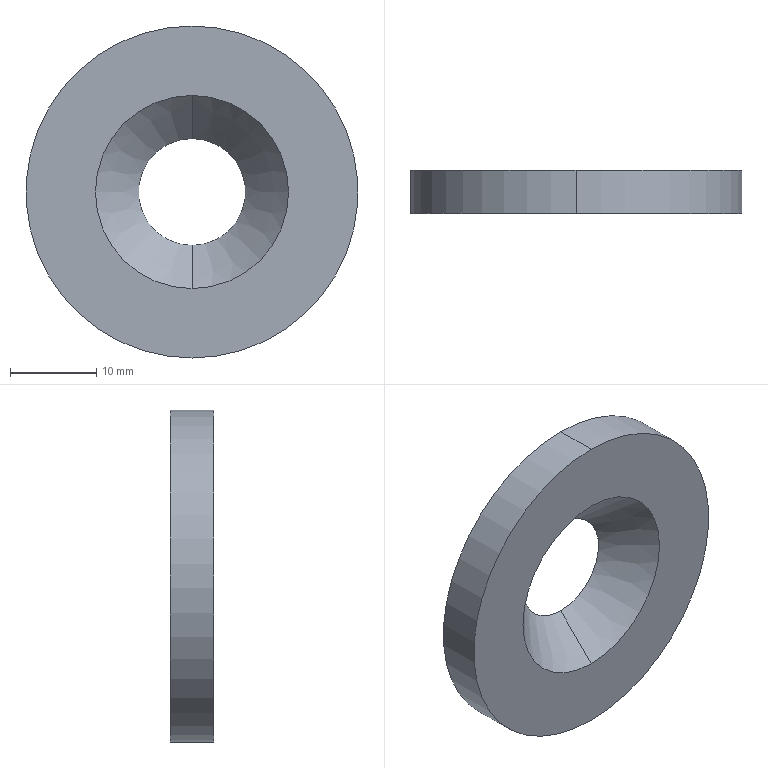Part | STEP file | PN_0018_default | 1 solid | 6 faces | box 38.5 x 5 x 38.5 mm | volume 4599 mm3 | cone 2 | cylinder 2 | plane 2 | commonest cylinder face diameters 38.5 x2
STEP:
#1=CARTESIAN_POINT('',(0.,0.,0.));
#2=DIRECTION('',(0.,0.,1.));
#3=DIRECTION('',(1.,0.,0.));
#4=AXIS2_PLACEMENT_3D('',#1,#2,#3);
#5=CARTESIAN_POINT('',(0.,5.,-6.2));
#6=VERTEX_POINT('',#5);
#7=CARTESIAN_POINT('',(0.,0.,-11.2));
#8=VERTEX_POINT('',#7);
#9=CARTESIAN_POINT('',(0.,0.,-11.2));
#10=DIRECTION('',(0.,-0.7071,-0.7071));
#11=VECTOR('',#10,1.);
#12=LINE('',#9,#11);
#13=CARTESIAN_POINT('',(0.,0.,0.));
#14=DIRECTION('',(0.,-1.,0.));
#15=DIRECTION('',(0.,0.,-1.));
#16=AXIS2_PLACEMENT_3D('',#13,#14,#15);
#17=CONICAL_SURFACE('',#16,11.2,0.7854);
#18=CARTESIAN_POINT('',(6.283,0.));
#19=DIRECTION('',(0.,1.));
#20=VECTOR('',#19,1.);
#21=LINE('',#18,#20);
#22=(GEOMETRIC_REPRESENTATION_CONTEXT(2)PARAMETRIC_REPRESENTATION_CONTEXT()REPRESENTATION_CONTEXT('',''));
#23=DEFINITIONAL_REPRESENTATION('',(#21),#22);
#24=PCURVE('',#17,#23);
#25=CARTESIAN_POINT('',(0.,0.,0.));
#26=DIRECTION('',(0.,-1.,0.));
#27=DIRECTION('',(0.,0.,-1.));
#28=AXIS2_PLACEMENT_3D('',#25,#26,#27);
#29=CONICAL_SURFACE('',#28,11.2,0.7854);
#30=CARTESIAN_POINT('',(0.,0.));
#31=DIRECTION('',(0.,1.));
#32=VECTOR('',#31,1.);
#33=LINE('',#30,#32);
#34=(GEOMETRIC_REPRESENTATION_CONTEXT(2)PARAMETRIC_REPRESENTATION_CONTEXT()REPRESENTATION_CONTEXT('',''));
#35=DEFINITIONAL_REPRESENTATION('',(#33),#34);
#36=PCURVE('',#29,#35);
#37=SURFACE_CURVE('',#12,(#24,#36),.PCURVE_S1.);
#38=EDGE_CURVE('',#6,#8,#37,.T.);
#39=ORIENTED_EDGE('',*,*,#38,.T.);
#40=CARTESIAN_POINT('',(0.,0.,11.2));
#41=VERTEX_POINT('',#40);
#42=CARTESIAN_POINT('',(0.,0.,0.));
#43=DIRECTION('',(0.,-1.,0.));
#44=DIRECTION('',(0.,0.,-1.));
#45=AXIS2_PLACEMENT_3D('',#42,#43,#44);
#46=CIRCLE('',#45,11.2);
#47=CARTESIAN_POINT('',(0.,0.));
#48=DIRECTION('',(1.,0.));
#49=VECTOR('',#48,1.);
#50=LINE('',#47,#49);
#51=(GEOMETRIC_REPRESENTATION_CONTEXT(2)PARAMETRIC_REPRESENTATION_CONTEXT()REPRESENTATION_CONTEXT('',''));
#52=DEFINITIONAL_REPRESENTATION('',(#50),#51);
#53=PCURVE('',#17,#52);
#54=CARTESIAN_POINT('',(0.,0.,0.));
#55=DIRECTION('',(0.,1.,0.));
#56=DIRECTION('',(0.,0.,1.));
#57=AXIS2_PLACEMENT_3D('',#54,#55,#56);
#58=PLANE('',#57);
#59=CARTESIAN_POINT('',(-11.2,0.));
#60=CARTESIAN_POINT('',(-11.2,19.399));
#61=CARTESIAN_POINT('',(5.6,9.699));
#62=CARTESIAN_POINT('',(22.4,0.));
#63=CARTESIAN_POINT('',(5.6,-9.699));
#64=CARTESIAN_POINT('',(-11.2,-19.399));
#65=CARTESIAN_POINT('',(-11.2,0.));
#66=(BOUNDED_CURVE()B_SPLINE_CURVE(2,(#59,#60,#61,#62,#63,#64,#65),.UNSPECIFIED.,.T.,.F.)B_SPLINE_CURVE_WITH_KNOTS((1,2,2,2,2,1),(-2.094,0.,2.094,4.189,6.283,8.378),.UNSPECIFIED.)CURVE()GEOMETRIC_REPRESENTATION_ITEM()RATIONAL_B_SPLINE_CURVE((1.,0.5,1.,0.5,1.,0.5,1.))REPRESENTATION_ITEM(''));
#67=(GEOMETRIC_REPRESENTATION_CONTEXT(2)PARAMETRIC_REPRESENTATION_CONTEXT()REPRESENTATION_CONTEXT('',''));
#68=DEFINITIONAL_REPRESENTATION('',(#66),#67);
#69=PCURVE('',#58,#68);
#70=SURFACE_CURVE('',#46,(#53,#69),.PCURVE_S1.);
#71=EDGE_CURVE('',#41,#8,#70,.T.);
#72=ORIENTED_EDGE('',*,*,#71,.F.);
#73=CARTESIAN_POINT('',(0.,5.,6.2));
#74=VERTEX_POINT('',#73);
#75=CARTESIAN_POINT('',(0.,0.,11.2));
#76=DIRECTION('',(0.,-0.7071,0.7071));
#77=VECTOR('',#76,1.);
#78=LINE('',#75,#77);
#79=CARTESIAN_POINT('',(3.142,0.));
#80=DIRECTION('',(0.,1.));
#81=VECTOR('',#80,1.);
#82=LINE('',#79,#81);
#83=(GEOMETRIC_REPRESENTATION_CONTEXT(2)PARAMETRIC_REPRESENTATION_CONTEXT()REPRESENTATION_CONTEXT('',''));
#84=DEFINITIONAL_REPRESENTATION('',(#82),#83);
#85=PCURVE('',#17,#84);
#86=CARTESIAN_POINT('',(3.142,0.));
#87=DIRECTION('',(0.,1.));
#88=VECTOR('',#87,1.);
#89=LINE('',#86,#88);
#90=(GEOMETRIC_REPRESENTATION_CONTEXT(2)PARAMETRIC_REPRESENTATION_CONTEXT()REPRESENTATION_CONTEXT('',''));
#91=DEFINITIONAL_REPRESENTATION('',(#89),#90);
#92=PCURVE('',#29,#91);
#93=SURFACE_CURVE('',#78,(#85,#92),.PCURVE_S1.);
#94=EDGE_CURVE('',#74,#41,#93,.T.);
#95=ORIENTED_EDGE('',*,*,#94,.F.);
#96=CARTESIAN_POINT('',(0.,5.,0.));
#97=DIRECTION('',(0.,1.,0.));
#98=DIRECTION('',(0.,0.,1.));
#99=AXIS2_PLACEMENT_3D('',#96,#97,#98);
#100=CIRCLE('',#99,6.2);
#101=CARTESIAN_POINT('',(9.425,-5.));
#102=DIRECTION('',(-1.,0.));
#103=VECTOR('',#102,1.);
#104=LINE('',#101,#103);
#105=(GEOMETRIC_REPRESENTATION_CONTEXT(2)PARAMETRIC_REPRESENTATION_CONTEXT()REPRESENTATION_CONTEXT('',''));
#106=DEFINITIONAL_REPRESENTATION('',(#104),#105);
#107=PCURVE('',#17,#106);
#108=CARTESIAN_POINT('',(0.,5.,0.));
#109=DIRECTION('',(0.,1.,0.));
#110=DIRECTION('',(0.,0.,1.));
#111=AXIS2_PLACEMENT_3D('',#108,#109,#110);
#112=PLANE('',#111);
#113=CARTESIAN_POINT('',(0.,0.));
#114=DIRECTION('',(1.,0.));
#115=AXIS2_PLACEMENT_2D('',#113,#114);
#116=CIRCLE('',#115,6.2);
#117=(GEOMETRIC_REPRESENTATION_CONTEXT(2)PARAMETRIC_REPRESENTATION_CONTEXT()REPRESENTATION_CONTEXT('',''));
#118=DEFINITIONAL_REPRESENTATION('',(#116),#117);
#119=PCURVE('',#112,#118);
#120=SURFACE_CURVE('',#100,(#107,#119),.PCURVE_S1.);
#121=EDGE_CURVE('',#6,#74,#120,.T.);
#122=ORIENTED_EDGE('',*,*,#121,.F.);
#123=EDGE_LOOP('',(#39,#72,#95,#122));
#124=FACE_BOUND('',#123,.F.);
#125=ADVANCED_FACE('',(#124),#17,.F.);
#126=CARTESIAN_POINT('',(0.,5.,19.25));
#127=VERTEX_POINT('',#126);
#128=CARTESIAN_POINT('',(0.,5.,-19.25));
#129=VERTEX_POINT('',#128);
#130=CARTESIAN_POINT('',(0.,5.,0.));
#131=DIRECTION('',(0.,1.,0.));
#132=DIRECTION('',(0.,0.,1.));
#133=AXIS2_PLACEMENT_3D('',#130,#131,#132);
#134=CIRCLE('',#133,19.25);
#135=CARTESIAN_POINT('',(0.,5.,0.));
#136=DIRECTION('',(0.,-1.,0.));
#137=DIRECTION('',(0.,0.,-1.));
#138=AXIS2_PLACEMENT_3D('',#135,#136,#137);
#139=CYLINDRICAL_SURFACE('',#138,19.25);
#140=CARTESIAN_POINT('',(3.142,0.));
#141=DIRECTION('',(-1.,0.));
#142=VECTOR('',#141,1.);
#143=LINE('',#140,#142);
#144=(GEOMETRIC_REPRESENTATION_CONTEXT(2)PARAMETRIC_REPRESENTATION_CONTEXT()REPRESENTATION_CONTEXT('',''));
#145=DEFINITIONAL_REPRESENTATION('',(#143),#144);
#146=PCURVE('',#139,#145);
#147=CARTESIAN_POINT('',(0.,0.));
#148=DIRECTION('',(1.,0.));
#149=AXIS2_PLACEMENT_2D('',#147,#148);
#150=CIRCLE('',#149,19.25);
#151=(GEOMETRIC_REPRESENTATION_CONTEXT(2)PARAMETRIC_REPRESENTATION_CONTEXT()REPRESENTATION_CONTEXT('',''));
#152=DEFINITIONAL_REPRESENTATION('',(#150),#151);
#153=PCURVE('',#112,#152);
#154=SURFACE_CURVE('',#134,(#146,#153),.PCURVE_S1.);
#155=EDGE_CURVE('',#127,#129,#154,.T.);
#156=ORIENTED_EDGE('',*,*,#155,.F.);
#157=CARTESIAN_POINT('',(0.,0.,19.25));
#158=VERTEX_POINT('',#157);
#159=CARTESIAN_POINT('',(0.,5.,19.25));
#160=DIRECTION('',(0.,-1.,0.));
#161=VECTOR('',#160,1.);
#162=LINE('',#159,#161);
#163=CARTESIAN_POINT('',(3.142,0.));
#164=DIRECTION('',(0.,1.));
#165=VECTOR('',#164,1.);
#166=LINE('',#163,#165);
#167=(GEOMETRIC_REPRESENTATION_CONTEXT(2)PARAMETRIC_REPRESENTATION_CONTEXT()REPRESENTATION_CONTEXT('',''));
#168=DEFINITIONAL_REPRESENTATION('',(#166),#167);
#169=PCURVE('',#139,#168);
#170=CARTESIAN_POINT('',(0.,5.,0.));
#171=DIRECTION('',(0.,-1.,0.));
#172=DIRECTION('',(0.,0.,-1.));
#173=AXIS2_PLACEMENT_3D('',#170,#171,#172);
#174=CYLINDRICAL_SURFACE('',#173,19.25);
#175=CARTESIAN_POINT('',(3.142,0.));
#176=DIRECTION('',(0.,1.));
#177=VECTOR('',#176,1.);
#178=LINE('',#175,#177);
#179=(GEOMETRIC_REPRESENTATION_CONTEXT(2)PARAMETRIC_REPRESENTATION_CONTEXT()REPRESENTATION_CONTEXT('',''));
#180=DEFINITIONAL_REPRESENTATION('',(#178),#179);
#181=PCURVE('',#174,#180);
#182=SURFACE_CURVE('',#162,(#169,#181),.PCURVE_S1.);
#183=EDGE_CURVE('',#127,#158,#182,.T.);
#184=ORIENTED_EDGE('',*,*,#183,.T.);
#185=CARTESIAN_POINT('',(0.,0.,-19.25));
#186=VERTEX_POINT('',#185);
#187=CARTESIAN_POINT('',(0.,0.,0.));
#188=DIRECTION('',(0.,1.,0.));
#189=DIRECTION('',(0.,0.,1.));
#190=AXIS2_PLACEMENT_3D('',#187,#188,#189);
#191=CIRCLE('',#190,19.25);
#192=CARTESIAN_POINT('',(3.142,5.));
#193=DIRECTION('',(-1.,0.));
#194=VECTOR('',#193,1.);
#195=LINE('',#192,#194);
#196=(GEOMETRIC_REPRESENTATION_CONTEXT(2)PARAMETRIC_REPRESENTATION_CONTEXT()REPRESENTATION_CONTEXT('',''));
#197=DEFINITIONAL_REPRESENTATION('',(#195),#196);
#198=PCURVE('',#139,#197);
#199=CARTESIAN_POINT('',(0.,0.));
#200=DIRECTION('',(1.,0.));
#201=AXIS2_PLACEMENT_2D('',#199,#200);
#202=CIRCLE('',#201,19.25);
#203=(GEOMETRIC_REPRESENTATION_CONTEXT(2)PARAMETRIC_REPRESENTATION_CONTEXT()REPRESENTATION_CONTEXT('',''));
#204=DEFINITIONAL_REPRESENTATION('',(#202),#203);
#205=PCURVE('',#58,#204);
#206=SURFACE_CURVE('',#191,(#198,#205),.PCURVE_S1.);
#207=EDGE_CURVE('',#158,#186,#206,.T.);
#208=ORIENTED_EDGE('',*,*,#207,.T.);
#209=CARTESIAN_POINT('',(0.,5.,-19.25));
#210=DIRECTION('',(0.,-1.,0.));
#211=VECTOR('',#210,1.);
#212=LINE('',#209,#211);
#213=CARTESIAN_POINT('',(0.,0.));
#214=DIRECTION('',(0.,1.));
#215=VECTOR('',#214,1.);
#216=LINE('',#213,#215);
#217=(GEOMETRIC_REPRESENTATION_CONTEXT(2)PARAMETRIC_REPRESENTATION_CONTEXT()REPRESENTATION_CONTEXT('',''));
#218=DEFINITIONAL_REPRESENTATION('',(#216),#217);
#219=PCURVE('',#139,#218);
#220=CARTESIAN_POINT('',(6.283,0.));
#221=DIRECTION('',(0.,1.));
#222=VECTOR('',#221,1.);
#223=LINE('',#220,#222);
#224=(GEOMETRIC_REPRESENTATION_CONTEXT(2)PARAMETRIC_REPRESENTATION_CONTEXT()REPRESENTATION_CONTEXT('',''));
#225=DEFINITIONAL_REPRESENTATION('',(#223),#224);
#226=PCURVE('',#174,#225);
#227=SURFACE_CURVE('',#212,(#219,#226),.PCURVE_S1.);
#228=EDGE_CURVE('',#129,#186,#227,.T.);
#229=ORIENTED_EDGE('',*,*,#228,.F.);
#230=EDGE_LOOP('',(#156,#184,#208,#229));
#231=FACE_BOUND('',#230,.T.);
#232=ADVANCED_FACE('',(#231),#139,.T.);
#233=ORIENTED_EDGE('',*,*,#121,.F.);
#234=CARTESIAN_POINT('',(0.,5.,0.));
#235=DIRECTION('',(0.,1.,0.));
#236=DIRECTION('',(0.,0.,1.));
#237=AXIS2_PLACEMENT_3D('',#234,#235,#236);
#238=CIRCLE('',#237,6.2);
#239=CARTESIAN_POINT('',(0.,0.));
#240=DIRECTION('',(1.,0.));
#241=AXIS2_PLACEMENT_2D('',#239,#240);
#242=CIRCLE('',#241,6.2);
#243=(GEOMETRIC_REPRESENTATION_CONTEXT(2)PARAMETRIC_REPRESENTATION_CONTEXT()REPRESENTATION_CONTEXT('',''));
#244=DEFINITIONAL_REPRESENTATION('',(#242),#243);
#245=PCURVE('',#112,#244);
#246=CARTESIAN_POINT('',(3.142,-5.));
#247=DIRECTION('',(-1.,0.));
#248=VECTOR('',#247,1.);
#249=LINE('',#246,#248);
#250=(GEOMETRIC_REPRESENTATION_CONTEXT(2)PARAMETRIC_REPRESENTATION_CONTEXT()REPRESENTATION_CONTEXT('',''));
#251=DEFINITIONAL_REPRESENTATION('',(#249),#250);
#252=PCURVE('',#29,#251);
#253=SURFACE_CURVE('',#238,(#245,#252),.PCURVE_S1.);
#254=EDGE_CURVE('',#74,#6,#253,.T.);
#255=ORIENTED_EDGE('',*,*,#254,.F.);
#256=EDGE_LOOP('',(#233,#255));
#257=FACE_BOUND('',#256,.T.);
#258=CARTESIAN_POINT('',(0.,5.,0.));
#259=DIRECTION('',(0.,1.,0.));
#260=DIRECTION('',(0.,0.,1.));
#261=AXIS2_PLACEMENT_3D('',#258,#259,#260);
#262=CIRCLE('',#261,19.25);
#263=CARTESIAN_POINT('',(0.,0.));
#264=DIRECTION('',(1.,0.));
#265=AXIS2_PLACEMENT_2D('',#263,#264);
#266=CIRCLE('',#265,19.25);
#267=(GEOMETRIC_REPRESENTATION_CONTEXT(2)PARAMETRIC_REPRESENTATION_CONTEXT()REPRESENTATION_CONTEXT('',''));
#268=DEFINITIONAL_REPRESENTATION('',(#266),#267);
#269=PCURVE('',#112,#268);
#270=CARTESIAN_POINT('',(9.425,0.));
#271=DIRECTION('',(-1.,0.));
#272=VECTOR('',#271,1.);
#273=LINE('',#270,#272);
#274=(GEOMETRIC_REPRESENTATION_CONTEXT(2)PARAMETRIC_REPRESENTATION_CONTEXT()REPRESENTATION_CONTEXT('',''));
#275=DEFINITIONAL_REPRESENTATION('',(#273),#274);
#276=PCURVE('',#174,#275);
#277=SURFACE_CURVE('',#262,(#269,#276),.PCURVE_S1.);
#278=EDGE_CURVE('',#129,#127,#277,.T.);
#279=ORIENTED_EDGE('',*,*,#278,.T.);
#280=ORIENTED_EDGE('',*,*,#155,.T.);
#281=EDGE_LOOP('',(#279,#280));
#282=FACE_BOUND('',#281,.T.);
#283=ADVANCED_FACE('',(#257,#282),#112,.T.);
#284=ORIENTED_EDGE('',*,*,#183,.F.);
#285=ORIENTED_EDGE('',*,*,#278,.F.);
#286=ORIENTED_EDGE('',*,*,#228,.T.);
#287=CARTESIAN_POINT('',(0.,0.,0.));
#288=DIRECTION('',(0.,1.,0.));
#289=DIRECTION('',(0.,0.,1.));
#290=AXIS2_PLACEMENT_3D('',#287,#288,#289);
#291=CIRCLE('',#290,19.25);
#292=CARTESIAN_POINT('',(9.425,5.));
#293=DIRECTION('',(-1.,0.));
#294=VECTOR('',#293,1.);
#295=LINE('',#292,#294);
#296=(GEOMETRIC_REPRESENTATION_CONTEXT(2)PARAMETRIC_REPRESENTATION_CONTEXT()REPRESENTATION_CONTEXT('',''));
#297=DEFINITIONAL_REPRESENTATION('',(#295),#296);
#298=PCURVE('',#174,#297);
#299=CARTESIAN_POINT('',(0.,0.));
#300=DIRECTION('',(1.,0.));
#301=AXIS2_PLACEMENT_2D('',#299,#300);
#302=CIRCLE('',#301,19.25);
#303=(GEOMETRIC_REPRESENTATION_CONTEXT(2)PARAMETRIC_REPRESENTATION_CONTEXT()REPRESENTATION_CONTEXT('',''));
#304=DEFINITIONAL_REPRESENTATION('',(#302),#303);
#305=PCURVE('',#58,#304);
#306=SURFACE_CURVE('',#291,(#298,#305),.PCURVE_S1.);
#307=EDGE_CURVE('',#186,#158,#306,.T.);
#308=ORIENTED_EDGE('',*,*,#307,.T.);
#309=EDGE_LOOP('',(#284,#285,#286,#308));
#310=FACE_BOUND('',#309,.T.);
#311=ADVANCED_FACE('',(#310),#174,.T.);
#312=CARTESIAN_POINT('',(0.,0.,0.));
#313=DIRECTION('',(0.,-1.,0.));
#314=DIRECTION('',(0.,0.,-1.));
#315=AXIS2_PLACEMENT_3D('',#312,#313,#314);
#316=CIRCLE('',#315,11.2);
#317=CARTESIAN_POINT('',(-11.2,0.));
#318=CARTESIAN_POINT('',(-11.2,19.399));
#319=CARTESIAN_POINT('',(5.6,9.699));
#320=CARTESIAN_POINT('',(22.4,0.));
#321=CARTESIAN_POINT('',(5.6,-9.699));
#322=CARTESIAN_POINT('',(-11.2,-19.399));
#323=CARTESIAN_POINT('',(-11.2,0.));
#324=(BOUNDED_CURVE()B_SPLINE_CURVE(2,(#317,#318,#319,#320,#321,#322,#323),.UNSPECIFIED.,.T.,.F.)B_SPLINE_CURVE_WITH_KNOTS((1,2,2,2,2,1),(-2.094,0.,2.094,4.189,6.283,8.378),.UNSPECIFIED.)CURVE()GEOMETRIC_REPRESENTATION_ITEM()RATIONAL_B_SPLINE_CURVE((1.,0.5,1.,0.5,1.,0.5,1.))REPRESENTATION_ITEM(''));
#325=(GEOMETRIC_REPRESENTATION_CONTEXT(2)PARAMETRIC_REPRESENTATION_CONTEXT()REPRESENTATION_CONTEXT('',''));
#326=DEFINITIONAL_REPRESENTATION('',(#324),#325);
#327=PCURVE('',#58,#326);
#328=CARTESIAN_POINT('',(0.,0.));
#329=DIRECTION('',(1.,0.));
#330=VECTOR('',#329,1.);
#331=LINE('',#328,#330);
#332=(GEOMETRIC_REPRESENTATION_CONTEXT(2)PARAMETRIC_REPRESENTATION_CONTEXT()REPRESENTATION_CONTEXT('',''));
#333=DEFINITIONAL_REPRESENTATION('',(#331),#332);
#334=PCURVE('',#29,#333);
#335=SURFACE_CURVE('',#316,(#327,#334),.PCURVE_S1.);
#336=EDGE_CURVE('',#8,#41,#335,.T.);
#337=ORIENTED_EDGE('',*,*,#336,.F.);
#338=ORIENTED_EDGE('',*,*,#71,.F.);
#339=EDGE_LOOP('',(#337,#338));
#340=FACE_BOUND('',#339,.T.);
#341=ORIENTED_EDGE('',*,*,#307,.F.);
#342=ORIENTED_EDGE('',*,*,#207,.F.);
#343=EDGE_LOOP('',(#341,#342));
#344=FACE_BOUND('',#343,.T.);
#345=ADVANCED_FACE('',(#340,#344),#58,.F.);
#346=ORIENTED_EDGE('',*,*,#336,.F.);
#347=ORIENTED_EDGE('',*,*,#38,.F.);
#348=ORIENTED_EDGE('',*,*,#254,.F.);
#349=ORIENTED_EDGE('',*,*,#94,.T.);
#350=EDGE_LOOP('',(#346,#347,#348,#349));
#351=FACE_BOUND('',#350,.F.);
#352=ADVANCED_FACE('',(#351),#29,.F.);
#353=CLOSED_SHELL('',(#125,#232,#283,#311,#345,#352));
#354=MANIFOLD_SOLID_BREP('',#353);
#355=(LENGTH_UNIT()NAMED_UNIT(*)SI_UNIT(.MILLI.,.METRE.));
#356=UNCERTAINTY_MEASURE_WITH_UNIT(LENGTH_MEASURE(0.0000001),#355,'','');
#357=(NAMED_UNIT(*)PLANE_ANGLE_UNIT()SI_UNIT($,.RADIAN.));
#358=(NAMED_UNIT(*)SI_UNIT($,.STERADIAN.)SOLID_ANGLE_UNIT());
#359=(GEOMETRIC_REPRESENTATION_CONTEXT(3)GLOBAL_UNCERTAINTY_ASSIGNED_CONTEXT((#356))GLOBAL_UNIT_ASSIGNED_CONTEXT((#355,#357,#358))REPRESENTATION_CONTEXT('',''));
#360=ADVANCED_BREP_SHAPE_REPRESENTATION('',(#4,#354),#359);